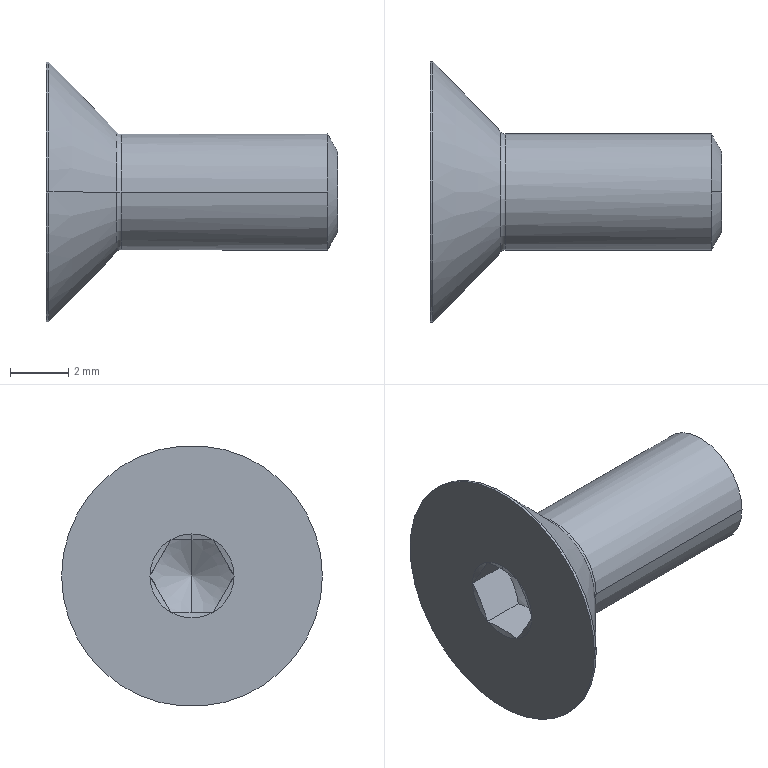Part | SolidWorks | features RevCut 2, Revolution 2, Cut 1, LPattern 1, RefAxis 1 | 1 solid | 27 faces | box 10 x 8.96 x 8.96 mm | volume 171.604 mm3 | cone 13 | plane 8 | cylinder 4 | torus 2 | commonest cylinder face diameters 4 x2 8.96 x2
STEP:
#1=CARTESIAN_POINT('',(0.,0.,1.394));
#2=VERTEX_POINT('',#1);
#3=CARTESIAN_POINT('',(0.,0.,-1.394));
#4=VERTEX_POINT('',#3);
#5=CARTESIAN_POINT('',(0.,0.,0.));
#6=DIRECTION('',(-1.,0.,0.));
#7=DIRECTION('',(0.,0.,1.));
#8=AXIS2_PLACEMENT_3D('',#5,#6,#7);
#9=CIRCLE('',#8,1.394);
#10=EDGE_CURVE('',#2,#4,#9,.T.);
#11=ORIENTED_EDGE('',*,*,#10,.T.);
#12=CARTESIAN_POINT('',(-0.35,0.,-2.));
#13=VERTEX_POINT('',#12);
#14=CARTESIAN_POINT('',(-0.35,0.,-2.));
#15=DIRECTION('',(-0.5,0.,-0.866));
#16=VECTOR('',#15,1000.);
#17=LINE('',#14,#16);
#18=EDGE_CURVE('',#4,#13,#17,.T.);
#19=ORIENTED_EDGE('',*,*,#18,.T.);
#20=CARTESIAN_POINT('',(-0.35,2.,0.));
#21=VERTEX_POINT('',#20);
#22=CARTESIAN_POINT('',(-0.35,0.,0.));
#23=DIRECTION('',(-1.,0.,0.));
#24=DIRECTION('',(0.,0.,1.));
#25=AXIS2_PLACEMENT_3D('',#22,#23,#24);
#26=CIRCLE('',#25,2.);
#27=EDGE_CURVE('',#21,#13,#26,.T.);
#28=ORIENTED_EDGE('',*,*,#27,.F.);
#29=CARTESIAN_POINT('',(-0.35,0.,2.));
#30=VERTEX_POINT('',#29);
#31=CARTESIAN_POINT('',(-0.35,0.,0.));
#32=DIRECTION('',(-1.,0.,0.));
#33=DIRECTION('',(0.,0.,1.));
#34=AXIS2_PLACEMENT_3D('',#31,#32,#33);
#35=CIRCLE('',#34,2.);
#36=EDGE_CURVE('',#30,#21,#35,.T.);
#37=ORIENTED_EDGE('',*,*,#36,.F.);
#38=CARTESIAN_POINT('',(-0.35,0.,2.));
#39=DIRECTION('',(-0.5,0.,0.866));
#40=VECTOR('',#39,1000.);
#41=LINE('',#38,#40);
#42=EDGE_CURVE('',#2,#30,#41,.T.);
#43=ORIENTED_EDGE('',*,*,#42,.F.);
#44=EDGE_LOOP('',(#11,#19,#28,#37,#43));
#45=FACE_OUTER_BOUND('',#44,.T.);
#46=CARTESIAN_POINT('',(-0.35,0.,0.));
#47=DIRECTION('',(-1.,0.,0.));
#48=DIRECTION('',(0.,0.,1.));
#49=AXIS2_PLACEMENT_3D('',#46,#47,#48);
#50=CONICAL_SURFACE('',#49,2.,1.047);
#51=ADVANCED_FACE('',(#45),#50,.T.);
#52=CARTESIAN_POINT('',(-7.667,0.,0.));
#53=VERTEX_POINT('',#52);
#54=CARTESIAN_POINT('',(-8.388,0.,1.25));
#55=VERTEX_POINT('',#54);
#56=CARTESIAN_POINT('',(-8.5,0.,1.443));
#57=DIRECTION('',(-0.5,0.,0.866));
#58=VECTOR('',#57,1000.);
#59=LINE('',#56,#58);
#60=EDGE_CURVE('',#53,#55,#59,.T.);
#61=ORIENTED_EDGE('',*,*,#60,.F.);
#62=CARTESIAN_POINT('',(-8.388,0.,-1.25));
#63=VERTEX_POINT('',#62);
#64=CARTESIAN_POINT('',(-8.5,0.,-1.443));
#65=DIRECTION('',(-0.5,0.,-0.866));
#66=VECTOR('',#65,1000.);
#67=LINE('',#64,#66);
#68=EDGE_CURVE('',#53,#63,#67,.T.);
#69=ORIENTED_EDGE('',*,*,#68,.T.);
#70=CARTESIAN_POINT('',(-8.5,-0.7217,-1.25));
#71=VERTEX_POINT('',#70);
#72=CARTESIAN_POINT('',(-8.388,0.,-1.25));
#73=CARTESIAN_POINT('',(-8.388,-0.2437,-1.25));
#74=CARTESIAN_POINT('',(-8.432,-0.4872,-1.25));
#75=CARTESIAN_POINT('',(-8.5,-0.7217,-1.25));
#76=B_SPLINE_CURVE_WITH_KNOTS('',3,(#72,#73,#74,#75),.UNSPECIFIED.,.F.,.F.,(4,4),(0.004596,0.005327),.UNSPECIFIED.);
#77=EDGE_CURVE('',#63,#71,#76,.T.);
#78=ORIENTED_EDGE('',*,*,#77,.T.);
#79=CARTESIAN_POINT('',(-8.5,-1.443,0.));
#80=VERTEX_POINT('',#79);
#81=CARTESIAN_POINT('',(-8.5,-0.7217,-1.25));
#82=CARTESIAN_POINT('',(-8.432,-0.8395,-1.046));
#83=CARTESIAN_POINT('',(-8.389,-0.9591,-0.8387));
#84=CARTESIAN_POINT('',(-8.388,-1.205,-0.4136));
#85=CARTESIAN_POINT('',(-8.432,-1.325,-0.2044));
#86=CARTESIAN_POINT('',(-8.5,-1.443,0.));
#87=B_SPLINE_CURVE_WITH_KNOTS('',3,(#81,#82,#83,#84,#85,#86),.UNSPECIFIED.,.F.,.F.,(4,2,4),(0.000000238,0.0007291,0.001458),.UNSPECIFIED.);
#88=EDGE_CURVE('',#71,#80,#87,.T.);
#89=ORIENTED_EDGE('',*,*,#88,.T.);
#90=CARTESIAN_POINT('',(-8.5,-0.7217,1.25));
#91=VERTEX_POINT('',#90);
#92=CARTESIAN_POINT('',(-8.5,-1.443,0.));
#93=CARTESIAN_POINT('',(-8.432,-1.326,0.2041));
#94=CARTESIAN_POINT('',(-8.389,-1.206,0.4113));
#95=CARTESIAN_POINT('',(-8.388,-0.9605,0.8364));
#96=CARTESIAN_POINT('',(-8.432,-0.8397,1.046));
#97=CARTESIAN_POINT('',(-8.5,-0.7217,1.25));
#98=B_SPLINE_CURVE_WITH_KNOTS('',3,(#92,#93,#94,#95,#96,#97),.UNSPECIFIED.,.F.,.F.,(4,2,4),(0.000000238,0.0007291,0.001458),.UNSPECIFIED.);
#99=EDGE_CURVE('',#80,#91,#98,.T.);
#100=ORIENTED_EDGE('',*,*,#99,.T.);
#101=CARTESIAN_POINT('',(-8.5,-0.7217,1.25));
#102=CARTESIAN_POINT('',(-8.432,-0.4872,1.25));
#103=CARTESIAN_POINT('',(-8.388,-0.2437,1.25));
#104=CARTESIAN_POINT('',(-8.388,0.,1.25));
#105=B_SPLINE_CURVE_WITH_KNOTS('',3,(#101,#102,#103,#104),.UNSPECIFIED.,.F.,.F.,(4,4),(0.001238,0.001967),.UNSPECIFIED.);
#106=EDGE_CURVE('',#91,#55,#105,.T.);
#107=ORIENTED_EDGE('',*,*,#106,.T.);
#108=EDGE_LOOP('',(#61,#69,#78,#89,#100,#107));
#109=FACE_OUTER_BOUND('',#108,.T.);
#110=CARTESIAN_POINT('',(-8.5,0.,0.));
#111=DIRECTION('',(-1.,0.,0.));
#112=DIRECTION('',(0.,0.,1.));
#113=AXIS2_PLACEMENT_3D('',#110,#111,#112);
#114=CONICAL_SURFACE('',#113,1.443,1.047);
#115=ADVANCED_FACE('',(#109),#114,.F.);
#116=CARTESIAN_POINT('',(-10.,0.7217,1.25));
#117=VERTEX_POINT('',#116);
#118=CARTESIAN_POINT('',(-9.945,0.,1.25));
#119=VERTEX_POINT('',#118);
#120=CARTESIAN_POINT('',(-10.,0.7217,1.25));
#121=CARTESIAN_POINT('',(-9.966,0.4817,1.25));
#122=CARTESIAN_POINT('',(-9.945,0.2412,1.25));
#123=CARTESIAN_POINT('',(-9.945,0.,1.25));
#124=B_SPLINE_CURVE_WITH_KNOTS('',3,(#120,#121,#122,#123),.UNSPECIFIED.,.F.,.F.,(4,4),(0.00303,0.003757),.UNSPECIFIED.);
#125=EDGE_CURVE('',#117,#119,#124,.T.);
#126=ORIENTED_EDGE('',*,*,#125,.T.);
#127=CARTESIAN_POINT('',(-10.,0.,1.443));
#128=VERTEX_POINT('',#127);
#129=CARTESIAN_POINT('',(-9.593,0.,0.));
#130=DIRECTION('',(-0.2714,0.,0.9625));
#131=VECTOR('',#130,1000.);
#132=LINE('',#129,#131);
#133=EDGE_CURVE('',#119,#128,#132,.T.);
#134=ORIENTED_EDGE('',*,*,#133,.T.);
#135=CARTESIAN_POINT('',(-10.,0.,0.));
#136=DIRECTION('',(1.,0.,0.));
#137=DIRECTION('',(0.,-1.,0.));
#138=AXIS2_PLACEMENT_3D('',#135,#136,#137);
#139=CIRCLE('',#138,1.443);
#140=EDGE_CURVE('',#117,#128,#139,.T.);
#141=ORIENTED_EDGE('',*,*,#140,.F.);
#142=EDGE_LOOP('',(#126,#134,#141));
#143=FACE_OUTER_BOUND('',#142,.T.);
#144=CARTESIAN_POINT('',(-1009.593,0.,0.));
#145=DIRECTION('',(-1.,0.,0.));
#146=DIRECTION('',(0.,0.,1.));
#147=AXIS2_PLACEMENT_3D('',#144,#145,#146);
#148=CONICAL_SURFACE('',#147,3546.378,1.296);
#149=ADVANCED_FACE('',(#143),#148,.F.);
#150=CARTESIAN_POINT('',(-7.435,-2.,0.));
#151=VERTEX_POINT('',#150);
#152=CARTESIAN_POINT('',(-7.435,2.,0.));
#153=VERTEX_POINT('',#152);
#154=CARTESIAN_POINT('',(-7.435,0.,0.));
#155=DIRECTION('',(1.,0.,0.));
#156=DIRECTION('',(0.,1.,0.));
#157=AXIS2_PLACEMENT_3D('',#154,#155,#156);
#158=CIRCLE('',#157,2.);
#159=EDGE_CURVE('',#151,#153,#158,.T.);
#160=ORIENTED_EDGE('',*,*,#159,.F.);
#161=CARTESIAN_POINT('',(-7.579,-2.061,0.));
#162=VERTEX_POINT('',#161);
#163=CARTESIAN_POINT('',(-7.435,-2.2,0.));
#164=DIRECTION('',(0.,0.,1.));
#165=DIRECTION('',(0.,-1.,0.));
#166=AXIS2_PLACEMENT_3D('',#163,#164,#165);
#167=CIRCLE('',#166,0.2);
#168=EDGE_CURVE('',#151,#162,#167,.T.);
#169=ORIENTED_EDGE('',*,*,#168,.T.);
#170=CARTESIAN_POINT('',(-7.579,2.061,0.));
#171=VERTEX_POINT('',#170);
#172=CARTESIAN_POINT('',(-7.579,0.,0.));
#173=DIRECTION('',(1.,0.,0.));
#174=DIRECTION('',(0.,1.,0.));
#175=AXIS2_PLACEMENT_3D('',#172,#173,#174);
#176=CIRCLE('',#175,2.061);
#177=EDGE_CURVE('',#162,#171,#176,.T.);
#178=ORIENTED_EDGE('',*,*,#177,.T.);
#179=CARTESIAN_POINT('',(-7.435,2.2,0.));
#180=DIRECTION('',(0.,0.,-1.));
#181=DIRECTION('',(-1.,0.,0.));
#182=AXIS2_PLACEMENT_3D('',#179,#180,#181);
#183=CIRCLE('',#182,0.2);
#184=EDGE_CURVE('',#153,#171,#183,.T.);
#185=ORIENTED_EDGE('',*,*,#184,.F.);
#186=EDGE_LOOP('',(#160,#169,#178,#185));
#187=FACE_OUTER_BOUND('',#186,.T.);
#188=CARTESIAN_POINT('',(-7.435,0.,0.));
#189=DIRECTION('',(1.,0.,0.));
#190=DIRECTION('',(0.,1.,0.));
#191=AXIS2_PLACEMENT_3D('',#188,#189,#190);
#192=TOROIDAL_SURFACE('',#191,2.2,0.2);
#193=ADVANCED_FACE('',(#187),#192,.F.);
#194=CARTESIAN_POINT('',(-7.579,0.,0.));
#195=DIRECTION('',(1.,0.,0.));
#196=DIRECTION('',(0.,1.,0.));
#197=AXIS2_PLACEMENT_3D('',#194,#195,#196);
#198=CIRCLE('',#197,2.061);
#199=EDGE_CURVE('',#171,#162,#198,.T.);
#200=ORIENTED_EDGE('',*,*,#199,.F.);
#201=CARTESIAN_POINT('',(-9.915,4.48,0.));
#202=VERTEX_POINT('',#201);
#203=CARTESIAN_POINT('',(-7.579,2.061,0.));
#204=DIRECTION('',(-0.6947,0.7193,0.));
#205=VECTOR('',#204,1000.);
#206=LINE('',#203,#205);
#207=EDGE_CURVE('',#171,#202,#206,.T.);
#208=ORIENTED_EDGE('',*,*,#207,.T.);
#209=CARTESIAN_POINT('',(-9.915,-4.48,0.));
#210=VERTEX_POINT('',#209);
#211=CARTESIAN_POINT('',(-9.915,0.,0.));
#212=DIRECTION('',(1.,0.,0.));
#213=DIRECTION('',(0.,1.,0.));
#214=AXIS2_PLACEMENT_3D('',#211,#212,#213);
#215=CIRCLE('',#214,4.48);
#216=EDGE_CURVE('',#202,#210,#215,.T.);
#217=ORIENTED_EDGE('',*,*,#216,.T.);
#218=CARTESIAN_POINT('',(-7.579,-2.061,0.));
#219=DIRECTION('',(-0.6947,-0.7193,0.));
#220=VECTOR('',#219,1000.);
#221=LINE('',#218,#220);
#222=EDGE_CURVE('',#162,#210,#221,.T.);
#223=ORIENTED_EDGE('',*,*,#222,.F.);
#224=EDGE_LOOP('',(#200,#208,#217,#223));
#225=FACE_OUTER_BOUND('',#224,.T.);
#226=CARTESIAN_POINT('',(-7.579,0.,0.));
#227=DIRECTION('',(-1.,0.,0.));
#228=DIRECTION('',(0.,-1.,0.));
#229=AXIS2_PLACEMENT_3D('',#226,#227,#228);
#230=CONICAL_SURFACE('',#229,2.061,0.8029);
#231=ADVANCED_FACE('',(#225),#230,.T.);
#232=CARTESIAN_POINT('',(-10.,4.48,0.));
#233=VERTEX_POINT('',#232);
#234=CARTESIAN_POINT('',(-10.,-4.48,0.));
#235=VERTEX_POINT('',#234);
#236=CARTESIAN_POINT('',(-10.,0.,0.));
#237=DIRECTION('',(1.,0.,0.));
#238=DIRECTION('',(0.,1.,0.));
#239=AXIS2_PLACEMENT_3D('',#236,#237,#238);
#240=CIRCLE('',#239,4.48);
#241=EDGE_CURVE('',#233,#235,#240,.T.);
#242=ORIENTED_EDGE('',*,*,#241,.T.);
#243=CARTESIAN_POINT('',(0.,-4.48,0.));
#244=DIRECTION('',(1.,0.,0.));
#245=VECTOR('',#244,1000.);
#246=LINE('',#243,#245);
#247=EDGE_CURVE('',#235,#210,#246,.T.);
#248=ORIENTED_EDGE('',*,*,#247,.T.);
#249=ORIENTED_EDGE('',*,*,#216,.F.);
#250=CARTESIAN_POINT('',(0.,4.48,0.));
#251=DIRECTION('',(1.,0.,0.));
#252=VECTOR('',#251,1000.);
#253=LINE('',#250,#252);
#254=EDGE_CURVE('',#233,#202,#253,.T.);
#255=ORIENTED_EDGE('',*,*,#254,.F.);
#256=EDGE_LOOP('',(#242,#248,#249,#255));
#257=FACE_OUTER_BOUND('',#256,.T.);
#258=CARTESIAN_POINT('',(0.,0.,0.));
#259=DIRECTION('',(1.,0.,0.));
#260=DIRECTION('',(0.,1.,0.));
#261=AXIS2_PLACEMENT_3D('',#258,#259,#260);
#262=CYLINDRICAL_SURFACE('',#261,4.48);
#263=ADVANCED_FACE('',(#257),#262,.T.);
#264=CARTESIAN_POINT('',(-7.435,0.,0.));
#265=DIRECTION('',(1.,0.,0.));
#266=DIRECTION('',(0.,1.,0.));
#267=AXIS2_PLACEMENT_3D('',#264,#265,#266);
#268=CIRCLE('',#267,2.);
#269=EDGE_CURVE('',#153,#151,#268,.T.);
#270=ORIENTED_EDGE('',*,*,#269,.T.);
#271=CARTESIAN_POINT('',(-0.35,-2.,0.));
#272=VERTEX_POINT('',#271);
#273=CARTESIAN_POINT('',(0.,-2.,0.));
#274=DIRECTION('',(1.,0.,0.));
#275=VECTOR('',#274,1000.);
#276=LINE('',#273,#275);
#277=EDGE_CURVE('',#151,#272,#276,.T.);
#278=ORIENTED_EDGE('',*,*,#277,.T.);
#279=CARTESIAN_POINT('',(-0.35,0.,0.));
#280=DIRECTION('',(-1.,0.,0.));
#281=DIRECTION('',(0.,0.,1.));
#282=AXIS2_PLACEMENT_3D('',#279,#280,#281);
#283=CIRCLE('',#282,2.);
#284=EDGE_CURVE('',#272,#30,#283,.T.);
#285=ORIENTED_EDGE('',*,*,#284,.T.);
#286=ORIENTED_EDGE('',*,*,#36,.T.);
#287=CARTESIAN_POINT('',(0.,2.,0.));
#288=DIRECTION('',(1.,0.,0.));
#289=VECTOR('',#288,1000.);
#290=LINE('',#287,#289);
#291=EDGE_CURVE('',#153,#21,#290,.T.);
#292=ORIENTED_EDGE('',*,*,#291,.F.);
#293=EDGE_LOOP('',(#270,#278,#285,#286,#292));
#294=FACE_OUTER_BOUND('',#293,.T.);
#295=CARTESIAN_POINT('',(0.,0.,0.));
#296=DIRECTION('',(1.,0.,0.));
#297=DIRECTION('',(0.,1.,0.));
#298=AXIS2_PLACEMENT_3D('',#295,#296,#297);
#299=CYLINDRICAL_SURFACE('',#298,2.);
#300=ADVANCED_FACE('',(#294),#299,.T.);
#301=ORIENTED_EDGE('',*,*,#277,.F.);
#302=ORIENTED_EDGE('',*,*,#159,.T.);
#303=ORIENTED_EDGE('',*,*,#291,.T.);
#304=ORIENTED_EDGE('',*,*,#27,.T.);
#305=CARTESIAN_POINT('',(-0.35,0.,0.));
#306=DIRECTION('',(-1.,0.,0.));
#307=DIRECTION('',(0.,0.,1.));
#308=AXIS2_PLACEMENT_3D('',#305,#306,#307);
#309=CIRCLE('',#308,2.);
#310=EDGE_CURVE('',#13,#272,#309,.T.);
#311=ORIENTED_EDGE('',*,*,#310,.T.);
#312=EDGE_LOOP('',(#301,#302,#303,#304,#311));
#313=FACE_OUTER_BOUND('',#312,.T.);
#314=CARTESIAN_POINT('',(0.,0.,0.));
#315=DIRECTION('',(1.,0.,0.));
#316=DIRECTION('',(0.,1.,0.));
#317=AXIS2_PLACEMENT_3D('',#314,#315,#316);
#318=CYLINDRICAL_SURFACE('',#317,2.);
#319=ADVANCED_FACE('',(#313),#318,.T.);
#320=ORIENTED_EDGE('',*,*,#241,.F.);
#321=CARTESIAN_POINT('',(-10.,0.,0.));
#322=DIRECTION('',(1.,0.,0.));
#323=DIRECTION('',(0.,1.,0.));
#324=AXIS2_PLACEMENT_3D('',#321,#322,#323);
#325=CIRCLE('',#324,4.48);
#326=EDGE_CURVE('',#235,#233,#325,.T.);
#327=ORIENTED_EDGE('',*,*,#326,.F.);
#328=EDGE_LOOP('',(#320,#327));
#329=FACE_OUTER_BOUND('',#328,.T.);
#330=CARTESIAN_POINT('',(-10.,-0.7217,1.25));
#331=VERTEX_POINT('',#330);
#332=CARTESIAN_POINT('',(-10.,-1.443,0.));
#333=VERTEX_POINT('',#332);
#334=CARTESIAN_POINT('',(-10.,0.,0.));
#335=DIRECTION('',(1.,0.,0.));
#336=DIRECTION('',(0.,-1.,0.));
#337=AXIS2_PLACEMENT_3D('',#334,#335,#336);
#338=CIRCLE('',#337,1.443);
#339=EDGE_CURVE('',#331,#333,#338,.T.);
#340=ORIENTED_EDGE('',*,*,#339,.T.);
#341=CARTESIAN_POINT('',(-10.,-0.7217,-1.25));
#342=VERTEX_POINT('',#341);
#343=CARTESIAN_POINT('',(-10.,0.,0.));
#344=DIRECTION('',(1.,0.,0.));
#345=DIRECTION('',(0.,-1.,0.));
#346=AXIS2_PLACEMENT_3D('',#343,#344,#345);
#347=CIRCLE('',#346,1.443);
#348=EDGE_CURVE('',#333,#342,#347,.T.);
#349=ORIENTED_EDGE('',*,*,#348,.T.);
#350=CARTESIAN_POINT('',(-10.,0.7217,-1.25));
#351=VERTEX_POINT('',#350);
#352=CARTESIAN_POINT('',(-10.,0.,0.));
#353=DIRECTION('',(1.,0.,0.));
#354=DIRECTION('',(0.,-1.,0.));
#355=AXIS2_PLACEMENT_3D('',#352,#353,#354);
#356=CIRCLE('',#355,1.443);
#357=EDGE_CURVE('',#342,#351,#356,.T.);
#358=ORIENTED_EDGE('',*,*,#357,.T.);
#359=CARTESIAN_POINT('',(-10.,1.443,0.));
#360=VERTEX_POINT('',#359);
#361=CARTESIAN_POINT('',(-10.,0.,0.));
#362=DIRECTION('',(1.,0.,0.));
#363=DIRECTION('',(0.,-1.,0.));
#364=AXIS2_PLACEMENT_3D('',#361,#362,#363);
#365=CIRCLE('',#364,1.443);
#366=EDGE_CURVE('',#351,#360,#365,.T.);
#367=ORIENTED_EDGE('',*,*,#366,.T.);
#368=CARTESIAN_POINT('',(-10.,0.,0.));
#369=DIRECTION('',(-1.,0.,0.));
#370=DIRECTION('',(0.,0.,1.));
#371=AXIS2_PLACEMENT_3D('',#368,#369,#370);
#372=CIRCLE('',#371,1.443);
#373=EDGE_CURVE('',#117,#360,#372,.T.);
#374=ORIENTED_EDGE('',*,*,#373,.F.);
#375=ORIENTED_EDGE('',*,*,#140,.T.);
#376=CARTESIAN_POINT('',(-10.,0.,0.));
#377=DIRECTION('',(1.,0.,0.));
#378=DIRECTION('',(0.,-1.,0.));
#379=AXIS2_PLACEMENT_3D('',#376,#377,#378);
#380=CIRCLE('',#379,1.443);
#381=EDGE_CURVE('',#128,#331,#380,.T.);
#382=ORIENTED_EDGE('',*,*,#381,.T.);
#383=EDGE_LOOP('',(#340,#349,#358,#367,#374,#375,#382));
#384=FACE_BOUND('',#383,.T.);
#385=CARTESIAN_POINT('',(-10.,4.48,0.));
#386=DIRECTION('',(-1.,0.,0.));
#387=DIRECTION('',(0.,-1.,0.));
#388=AXIS2_PLACEMENT_3D('',#385,#386,#387);
#389=PLANE('',#388);
#390=ADVANCED_FACE('',(#329,#384),#389,.T.);
#391=ORIENTED_EDGE('',*,*,#247,.F.);
#392=ORIENTED_EDGE('',*,*,#326,.T.);
#393=ORIENTED_EDGE('',*,*,#254,.T.);
#394=CARTESIAN_POINT('',(-9.915,0.,0.));
#395=DIRECTION('',(1.,0.,0.));
#396=DIRECTION('',(0.,1.,0.));
#397=AXIS2_PLACEMENT_3D('',#394,#395,#396);
#398=CIRCLE('',#397,4.48);
#399=EDGE_CURVE('',#210,#202,#398,.T.);
#400=ORIENTED_EDGE('',*,*,#399,.F.);
#401=EDGE_LOOP('',(#391,#392,#393,#400));
#402=FACE_OUTER_BOUND('',#401,.T.);
#403=CARTESIAN_POINT('',(0.,0.,0.));
#404=DIRECTION('',(1.,0.,0.));
#405=DIRECTION('',(0.,1.,0.));
#406=AXIS2_PLACEMENT_3D('',#403,#404,#405);
#407=CYLINDRICAL_SURFACE('',#406,4.48);
#408=ADVANCED_FACE('',(#402),#407,.T.);
#409=ORIENTED_EDGE('',*,*,#207,.F.);
#410=ORIENTED_EDGE('',*,*,#177,.F.);
#411=ORIENTED_EDGE('',*,*,#222,.T.);
#412=ORIENTED_EDGE('',*,*,#399,.T.);
#413=EDGE_LOOP('',(#409,#410,#411,#412));
#414=FACE_OUTER_BOUND('',#413,.T.);
#415=CARTESIAN_POINT('',(-7.579,0.,0.));
#416=DIRECTION('',(-1.,0.,0.));
#417=DIRECTION('',(0.,-1.,0.));
#418=AXIS2_PLACEMENT_3D('',#415,#416,#417);
#419=CONICAL_SURFACE('',#418,2.061,0.8029);
#420=ADVANCED_FACE('',(#414),#419,.T.);
#421=ORIENTED_EDGE('',*,*,#168,.F.);
#422=ORIENTED_EDGE('',*,*,#269,.F.);
#423=ORIENTED_EDGE('',*,*,#184,.T.);
#424=ORIENTED_EDGE('',*,*,#199,.T.);
#425=EDGE_LOOP('',(#421,#422,#423,#424));
#426=FACE_OUTER_BOUND('',#425,.T.);
#427=CARTESIAN_POINT('',(-7.435,0.,0.));
#428=DIRECTION('',(1.,0.,0.));
#429=DIRECTION('',(0.,1.,0.));
#430=AXIS2_PLACEMENT_3D('',#427,#428,#429);
#431=TOROIDAL_SURFACE('',#430,2.2,0.2);
#432=ADVANCED_FACE('',(#426),#431,.F.);
#433=CARTESIAN_POINT('',(-10.,-0.7217,1.25));
#434=CARTESIAN_POINT('',(-9.966,-0.842,1.042));
#435=CARTESIAN_POINT('',(-9.925,-1.083,0.625));
#436=CARTESIAN_POINT('',(-9.966,-1.323,0.2083));
#437=CARTESIAN_POINT('',(-10.,-1.443,0.));
#438=B_SPLINE_CURVE_WITH_KNOTS('',3,(#433,#434,#435,#436,#437),.UNSPECIFIED.,.F.,.F.,(4,1,4),(0.000000231,0.0007219,0.001444),.UNSPECIFIED.);
#439=EDGE_CURVE('',#331,#333,#438,.T.);
#440=ORIENTED_EDGE('',*,*,#439,.T.);
#441=ORIENTED_EDGE('',*,*,#339,.F.);
#442=EDGE_LOOP('',(#440,#441));
#443=FACE_OUTER_BOUND('',#442,.T.);
#444=CARTESIAN_POINT('',(-1009.593,0.,0.));
#445=DIRECTION('',(-1.,0.,0.));
#446=DIRECTION('',(0.,0.,1.));
#447=AXIS2_PLACEMENT_3D('',#444,#445,#446);
#448=CONICAL_SURFACE('',#447,3546.378,1.296);
#449=ADVANCED_FACE('',(#443),#448,.F.);
#450=ORIENTED_EDGE('',*,*,#133,.F.);
#451=CARTESIAN_POINT('',(-9.945,0.,1.25));
#452=CARTESIAN_POINT('',(-9.945,-0.2402,1.25));
#453=CARTESIAN_POINT('',(-9.966,-0.482,1.25));
#454=CARTESIAN_POINT('',(-10.,-0.7217,1.25));
#455=B_SPLINE_CURVE_WITH_KNOTS('',3,(#451,#452,#453,#454),.UNSPECIFIED.,.F.,.F.,(4,4),(0.003757,0.004481),.UNSPECIFIED.);
#456=EDGE_CURVE('',#119,#331,#455,.T.);
#457=ORIENTED_EDGE('',*,*,#456,.T.);
#458=ORIENTED_EDGE('',*,*,#381,.F.);
#459=EDGE_LOOP('',(#450,#457,#458));
#460=FACE_OUTER_BOUND('',#459,.T.);
#461=CARTESIAN_POINT('',(-1009.593,0.,0.));
#462=DIRECTION('',(-1.,0.,0.));
#463=DIRECTION('',(0.,0.,1.));
#464=AXIS2_PLACEMENT_3D('',#461,#462,#463);
#465=CONICAL_SURFACE('',#464,3546.378,1.296);
#466=ADVANCED_FACE('',(#460),#465,.F.);
#467=CARTESIAN_POINT('',(-10.,1.443,0.));
#468=CARTESIAN_POINT('',(-9.966,1.323,0.2083));
#469=CARTESIAN_POINT('',(-9.925,1.083,0.625));
#470=CARTESIAN_POINT('',(-9.966,0.842,1.042));
#471=CARTESIAN_POINT('',(-10.,0.7217,1.25));
#472=B_SPLINE_CURVE_WITH_KNOTS('',3,(#467,#468,#469,#470,#471),.UNSPECIFIED.,.F.,.F.,(4,1,4),(0.000000231,0.0007219,0.001444),.UNSPECIFIED.);
#473=EDGE_CURVE('',#360,#117,#472,.T.);
#474=ORIENTED_EDGE('',*,*,#473,.T.);
#475=ORIENTED_EDGE('',*,*,#373,.T.);
#476=EDGE_LOOP('',(#474,#475));
#477=FACE_OUTER_BOUND('',#476,.T.);
#478=CARTESIAN_POINT('',(-1009.593,0.,0.));
#479=DIRECTION('',(-1.,0.,0.));
#480=DIRECTION('',(0.,0.,1.));
#481=AXIS2_PLACEMENT_3D('',#478,#479,#480);
#482=CONICAL_SURFACE('',#481,3546.378,1.296);
#483=ADVANCED_FACE('',(#477),#482,.F.);
#484=CARTESIAN_POINT('',(-10.,0.7217,-1.25));
#485=CARTESIAN_POINT('',(-9.966,0.842,-1.042));
#486=CARTESIAN_POINT('',(-9.925,1.083,-0.625));
#487=CARTESIAN_POINT('',(-9.966,1.323,-0.2083));
#488=CARTESIAN_POINT('',(-10.,1.443,0.));
#489=B_SPLINE_CURVE_WITH_KNOTS('',3,(#484,#485,#486,#487,#488),.UNSPECIFIED.,.F.,.F.,(4,1,4),(0.000000231,0.0007219,0.001444),.UNSPECIFIED.);
#490=EDGE_CURVE('',#351,#360,#489,.T.);
#491=ORIENTED_EDGE('',*,*,#490,.T.);
#492=ORIENTED_EDGE('',*,*,#366,.F.);
#493=EDGE_LOOP('',(#491,#492));
#494=FACE_OUTER_BOUND('',#493,.T.);
#495=CARTESIAN_POINT('',(-1009.593,0.,0.));
#496=DIRECTION('',(-1.,0.,0.));
#497=DIRECTION('',(0.,0.,1.));
#498=AXIS2_PLACEMENT_3D('',#495,#496,#497);
#499=CONICAL_SURFACE('',#498,3546.378,1.296);
#500=ADVANCED_FACE('',(#494),#499,.F.);
#501=CARTESIAN_POINT('',(-10.,-0.7217,-1.25));
#502=CARTESIAN_POINT('',(-9.966,-0.4815,-1.25));
#503=CARTESIAN_POINT('',(-9.945,-0.2392,-1.25));
#504=CARTESIAN_POINT('',(-9.946,0.2422,-1.25));
#505=CARTESIAN_POINT('',(-9.966,0.4822,-1.25));
#506=CARTESIAN_POINT('',(-10.,0.7217,-1.25));
#507=B_SPLINE_CURVE_WITH_KNOTS('',3,(#501,#502,#503,#504,#505,#506),.UNSPECIFIED.,.F.,.F.,(4,2,4),(0.001183,0.00191,0.002636),.UNSPECIFIED.);
#508=EDGE_CURVE('',#342,#351,#507,.T.);
#509=ORIENTED_EDGE('',*,*,#508,.T.);
#510=ORIENTED_EDGE('',*,*,#357,.F.);
#511=EDGE_LOOP('',(#509,#510));
#512=FACE_OUTER_BOUND('',#511,.T.);
#513=CARTESIAN_POINT('',(-1009.593,0.,0.));
#514=DIRECTION('',(-1.,0.,0.));
#515=DIRECTION('',(0.,0.,1.));
#516=AXIS2_PLACEMENT_3D('',#513,#514,#515);
#517=CONICAL_SURFACE('',#516,3546.378,1.296);
#518=ADVANCED_FACE('',(#512),#517,.F.);
#519=CARTESIAN_POINT('',(-10.,-1.443,0.));
#520=CARTESIAN_POINT('',(-9.966,-1.323,-0.2083));
#521=CARTESIAN_POINT('',(-9.925,-1.083,-0.625));
#522=CARTESIAN_POINT('',(-9.966,-0.842,-1.042));
#523=CARTESIAN_POINT('',(-10.,-0.7217,-1.25));
#524=B_SPLINE_CURVE_WITH_KNOTS('',3,(#519,#520,#521,#522,#523),.UNSPECIFIED.,.F.,.F.,(4,1,4),(0.000000231,0.0007219,0.001444),.UNSPECIFIED.);
#525=EDGE_CURVE('',#333,#342,#524,.T.);
#526=ORIENTED_EDGE('',*,*,#525,.T.);
#527=ORIENTED_EDGE('',*,*,#348,.F.);
#528=EDGE_LOOP('',(#526,#527));
#529=FACE_OUTER_BOUND('',#528,.T.);
#530=CARTESIAN_POINT('',(-1009.593,0.,0.));
#531=DIRECTION('',(-1.,0.,0.));
#532=DIRECTION('',(0.,0.,1.));
#533=AXIS2_PLACEMENT_3D('',#530,#531,#532);
#534=CONICAL_SURFACE('',#533,3546.378,1.296);
#535=ADVANCED_FACE('',(#529),#534,.F.);
#536=ORIENTED_EDGE('',*,*,#68,.F.);
#537=ORIENTED_EDGE('',*,*,#60,.T.);
#538=CARTESIAN_POINT('',(-8.5,0.7217,1.25));
#539=VERTEX_POINT('',#538);
#540=CARTESIAN_POINT('',(-8.388,0.,1.25));
#541=CARTESIAN_POINT('',(-8.388,0.1219,1.25));
#542=CARTESIAN_POINT('',(-8.399,0.2454,1.25));
#543=CARTESIAN_POINT('',(-8.438,0.4868,1.25));
#544=CARTESIAN_POINT('',(-8.466,0.605,1.25));
#545=CARTESIAN_POINT('',(-8.5,0.7217,1.25));
#546=B_SPLINE_CURVE_WITH_KNOTS('',3,(#540,#541,#542,#543,#544,#545),.UNSPECIFIED.,.F.,.F.,(4,2,4),(0.001967,0.002332,0.002697),.UNSPECIFIED.);
#547=EDGE_CURVE('',#55,#539,#546,.T.);
#548=ORIENTED_EDGE('',*,*,#547,.T.);
#549=CARTESIAN_POINT('',(-8.5,1.443,0.));
#550=VERTEX_POINT('',#549);
#551=CARTESIAN_POINT('',(-8.5,0.7217,1.25));
#552=CARTESIAN_POINT('',(-8.432,0.8395,1.046));
#553=CARTESIAN_POINT('',(-8.389,0.9591,0.8387));
#554=CARTESIAN_POINT('',(-8.388,1.205,0.4136));
#555=CARTESIAN_POINT('',(-8.432,1.325,0.2044));
#556=CARTESIAN_POINT('',(-8.5,1.443,0.));
#557=B_SPLINE_CURVE_WITH_KNOTS('',3,(#551,#552,#553,#554,#555,#556),.UNSPECIFIED.,.F.,.F.,(4,2,4),(0.000000238,0.0007291,0.001458),.UNSPECIFIED.);
#558=EDGE_CURVE('',#539,#550,#557,.T.);
#559=ORIENTED_EDGE('',*,*,#558,.T.);
#560=CARTESIAN_POINT('',(-8.5,0.7217,-1.25));
#561=VERTEX_POINT('',#560);
#562=CARTESIAN_POINT('',(-8.5,1.443,0.));
#563=CARTESIAN_POINT('',(-8.432,1.326,-0.2041));
#564=CARTESIAN_POINT('',(-8.389,1.206,-0.4113));
#565=CARTESIAN_POINT('',(-8.388,0.9605,-0.8364));
#566=CARTESIAN_POINT('',(-8.432,0.8397,-1.046));
#567=CARTESIAN_POINT('',(-8.5,0.7217,-1.25));
#568=B_SPLINE_CURVE_WITH_KNOTS('',3,(#562,#563,#564,#565,#566,#567),.UNSPECIFIED.,.F.,.F.,(4,2,4),(0.000000238,0.0007291,0.001458),.UNSPECIFIED.);
#569=EDGE_CURVE('',#550,#561,#568,.T.);
#570=ORIENTED_EDGE('',*,*,#569,.T.);
#571=CARTESIAN_POINT('',(-8.5,0.7217,-1.25));
#572=CARTESIAN_POINT('',(-8.466,0.605,-1.25));
#573=CARTESIAN_POINT('',(-8.438,0.4868,-1.25));
#574=CARTESIAN_POINT('',(-8.399,0.2454,-1.25));
#575=CARTESIAN_POINT('',(-8.388,0.1219,-1.25));
#576=CARTESIAN_POINT('',(-8.388,0.,-1.25));
#577=B_SPLINE_CURVE_WITH_KNOTS('',3,(#571,#572,#573,#574,#575,#576),.UNSPECIFIED.,.F.,.F.,(4,2,4),(0.003865,0.004231,0.004596),.UNSPECIFIED.);
#578=EDGE_CURVE('',#561,#63,#577,.T.);
#579=ORIENTED_EDGE('',*,*,#578,.T.);
#580=EDGE_LOOP('',(#536,#537,#548,#559,#570,#579));
#581=FACE_OUTER_BOUND('',#580,.T.);
#582=CARTESIAN_POINT('',(-8.5,0.,0.));
#583=DIRECTION('',(-1.,0.,0.));
#584=DIRECTION('',(0.,0.,1.));
#585=AXIS2_PLACEMENT_3D('',#582,#583,#584);
#586=CONICAL_SURFACE('',#585,1.443,1.047);
#587=ADVANCED_FACE('',(#581),#586,.F.);
#588=ORIENTED_EDGE('',*,*,#490,.F.);
#589=CARTESIAN_POINT('',(-7.42,0.7217,-1.25));
#590=DIRECTION('',(-1.,0.,0.));
#591=VECTOR('',#590,1000.);
#592=LINE('',#589,#591);
#593=EDGE_CURVE('',#561,#351,#592,.T.);
#594=ORIENTED_EDGE('',*,*,#593,.F.);
#595=ORIENTED_EDGE('',*,*,#569,.F.);
#596=CARTESIAN_POINT('',(-7.42,1.443,0.));
#597=DIRECTION('',(-1.,0.,0.));
#598=VECTOR('',#597,1000.);
#599=LINE('',#596,#598);
#600=EDGE_CURVE('',#550,#360,#599,.T.);
#601=ORIENTED_EDGE('',*,*,#600,.T.);
#602=EDGE_LOOP('',(#588,#594,#595,#601));
#603=FACE_OUTER_BOUND('',#602,.T.);
#604=CARTESIAN_POINT('',(-7.42,1.443,0.));
#605=DIRECTION('',(0.,0.866,-0.5));
#606=DIRECTION('',(0.,0.5,0.866));
#607=AXIS2_PLACEMENT_3D('',#604,#605,#606);
#608=PLANE('',#607);
#609=ADVANCED_FACE('',(#603),#608,.F.);
#610=ORIENTED_EDGE('',*,*,#508,.F.);
#611=CARTESIAN_POINT('',(-7.42,-0.7217,-1.25));
#612=DIRECTION('',(-1.,0.,0.));
#613=VECTOR('',#612,1000.);
#614=LINE('',#611,#613);
#615=EDGE_CURVE('',#71,#342,#614,.T.);
#616=ORIENTED_EDGE('',*,*,#615,.F.);
#617=ORIENTED_EDGE('',*,*,#77,.F.);
#618=ORIENTED_EDGE('',*,*,#578,.F.);
#619=ORIENTED_EDGE('',*,*,#593,.T.);
#620=EDGE_LOOP('',(#610,#616,#617,#618,#619));
#621=FACE_OUTER_BOUND('',#620,.T.);
#622=CARTESIAN_POINT('',(-7.42,0.7217,-1.25));
#623=DIRECTION('',(0.,0.,-1.));
#624=DIRECTION('',(-1.,0.,0.));
#625=AXIS2_PLACEMENT_3D('',#622,#623,#624);
#626=PLANE('',#625);
#627=ADVANCED_FACE('',(#621),#626,.F.);
#628=ORIENTED_EDGE('',*,*,#525,.F.);
#629=CARTESIAN_POINT('',(-7.42,-1.443,0.));
#630=DIRECTION('',(-1.,0.,0.));
#631=VECTOR('',#630,1000.);
#632=LINE('',#629,#631);
#633=EDGE_CURVE('',#80,#333,#632,.T.);
#634=ORIENTED_EDGE('',*,*,#633,.F.);
#635=ORIENTED_EDGE('',*,*,#88,.F.);
#636=ORIENTED_EDGE('',*,*,#615,.T.);
#637=EDGE_LOOP('',(#628,#634,#635,#636));
#638=FACE_OUTER_BOUND('',#637,.T.);
#639=CARTESIAN_POINT('',(-7.42,-0.7217,-1.25));
#640=DIRECTION('',(0.,-0.866,-0.5));
#641=DIRECTION('',(0.,0.5,-0.866));
#642=AXIS2_PLACEMENT_3D('',#639,#640,#641);
#643=PLANE('',#642);
#644=ADVANCED_FACE('',(#638),#643,.F.);
#645=ORIENTED_EDGE('',*,*,#439,.F.);
#646=CARTESIAN_POINT('',(-7.42,-0.7217,1.25));
#647=DIRECTION('',(-1.,0.,0.));
#648=VECTOR('',#647,1000.);
#649=LINE('',#646,#648);
#650=EDGE_CURVE('',#91,#331,#649,.T.);
#651=ORIENTED_EDGE('',*,*,#650,.F.);
#652=ORIENTED_EDGE('',*,*,#99,.F.);
#653=ORIENTED_EDGE('',*,*,#633,.T.);
#654=EDGE_LOOP('',(#645,#651,#652,#653));
#655=FACE_OUTER_BOUND('',#654,.T.);
#656=CARTESIAN_POINT('',(-7.42,-1.443,0.));
#657=DIRECTION('',(0.,-0.866,0.5));
#658=DIRECTION('',(0.,-0.5,-0.866));
#659=AXIS2_PLACEMENT_3D('',#656,#657,#658);
#660=PLANE('',#659);
#661=ADVANCED_FACE('',(#655),#660,.F.);
#662=ORIENTED_EDGE('',*,*,#125,.F.);
#663=CARTESIAN_POINT('',(-7.42,0.7217,1.25));
#664=DIRECTION('',(-1.,0.,0.));
#665=VECTOR('',#664,1000.);
#666=LINE('',#663,#665);
#667=EDGE_CURVE('',#539,#117,#666,.T.);
#668=ORIENTED_EDGE('',*,*,#667,.F.);
#669=ORIENTED_EDGE('',*,*,#547,.F.);
#670=ORIENTED_EDGE('',*,*,#106,.F.);
#671=ORIENTED_EDGE('',*,*,#650,.T.);
#672=ORIENTED_EDGE('',*,*,#456,.F.);
#673=EDGE_LOOP('',(#662,#668,#669,#670,#671,#672));
#674=FACE_OUTER_BOUND('',#673,.T.);
#675=CARTESIAN_POINT('',(-7.42,-0.7217,1.25));
#676=DIRECTION('',(0.,0.,1.));
#677=DIRECTION('',(0.,-1.,0.));
#678=AXIS2_PLACEMENT_3D('',#675,#676,#677);
#679=PLANE('',#678);
#680=ADVANCED_FACE('',(#674),#679,.F.);
#681=ORIENTED_EDGE('',*,*,#473,.F.);
#682=ORIENTED_EDGE('',*,*,#600,.F.);
#683=ORIENTED_EDGE('',*,*,#558,.F.);
#684=ORIENTED_EDGE('',*,*,#667,.T.);
#685=EDGE_LOOP('',(#681,#682,#683,#684));
#686=FACE_OUTER_BOUND('',#685,.T.);
#687=CARTESIAN_POINT('',(-7.42,0.7217,1.25));
#688=DIRECTION('',(0.,0.866,0.5));
#689=DIRECTION('',(0.,-0.5,0.866));
#690=AXIS2_PLACEMENT_3D('',#687,#688,#689);
#691=PLANE('',#690);
#692=ADVANCED_FACE('',(#686),#691,.F.);
#693=ORIENTED_EDGE('',*,*,#18,.F.);
#694=CARTESIAN_POINT('',(0.,0.,0.));
#695=DIRECTION('',(-1.,0.,0.));
#696=DIRECTION('',(0.,0.,1.));
#697=AXIS2_PLACEMENT_3D('',#694,#695,#696);
#698=CIRCLE('',#697,1.394);
#699=EDGE_CURVE('',#4,#2,#698,.T.);
#700=ORIENTED_EDGE('',*,*,#699,.T.);
#701=ORIENTED_EDGE('',*,*,#42,.T.);
#702=ORIENTED_EDGE('',*,*,#284,.F.);
#703=ORIENTED_EDGE('',*,*,#310,.F.);
#704=EDGE_LOOP('',(#693,#700,#701,#702,#703));
#705=FACE_OUTER_BOUND('',#704,.T.);
#706=CARTESIAN_POINT('',(-0.35,0.,0.));
#707=DIRECTION('',(-1.,0.,0.));
#708=DIRECTION('',(0.,0.,1.));
#709=AXIS2_PLACEMENT_3D('',#706,#707,#708);
#710=CONICAL_SURFACE('',#709,2.,1.047);
#711=ADVANCED_FACE('',(#705),#710,.T.);
#712=ORIENTED_EDGE('',*,*,#10,.F.);
#713=ORIENTED_EDGE('',*,*,#699,.F.);
#714=EDGE_LOOP('',(#712,#713));
#715=FACE_OUTER_BOUND('',#714,.T.);
#716=CARTESIAN_POINT('',(0.,0.,0.));
#717=DIRECTION('',(1.,0.,0.));
#718=DIRECTION('',(0.,1.,0.));
#719=AXIS2_PLACEMENT_3D('',#716,#717,#718);
#720=PLANE('',#719);
#721=ADVANCED_FACE('',(#715),#720,.T.);
#722=CLOSED_SHELL('',(#51,#115,#149,#193,#231,#263,#300,#319,#390,#408,#420,#432,#449,#466,#483,#500,#518,#535,#587,#609,#627,#644,#661,#680,#692,#711,#721));
#723=MANIFOLD_SOLID_BREP('',#722);
#724=CARTESIAN_POINT('',(0.,0.,0.));
#725=DIRECTION('',(0.,0.,1.));
#726=DIRECTION('',(1.,0.,0.));
#727=AXIS2_PLACEMENT_3D('',#724,#725,#726);
#728=(LENGTH_UNIT()NAMED_UNIT(*)SI_UNIT(.MILLI.,.METRE.));
#729=UNCERTAINTY_MEASURE_WITH_UNIT(LENGTH_MEASURE(0.00001),#728,'','');
#730=(NAMED_UNIT(*)PLANE_ANGLE_UNIT()SI_UNIT($,.RADIAN.));
#731=(NAMED_UNIT(*)SI_UNIT($,.STERADIAN.)SOLID_ANGLE_UNIT());
#732=(GEOMETRIC_REPRESENTATION_CONTEXT(3)GLOBAL_UNCERTAINTY_ASSIGNED_CONTEXT((#729))GLOBAL_UNIT_ASSIGNED_CONTEXT((#728,#730,#731))REPRESENTATION_CONTEXT('',''));
#733=ADVANCED_BREP_SHAPE_REPRESENTATION('',(#723,#727),#732);